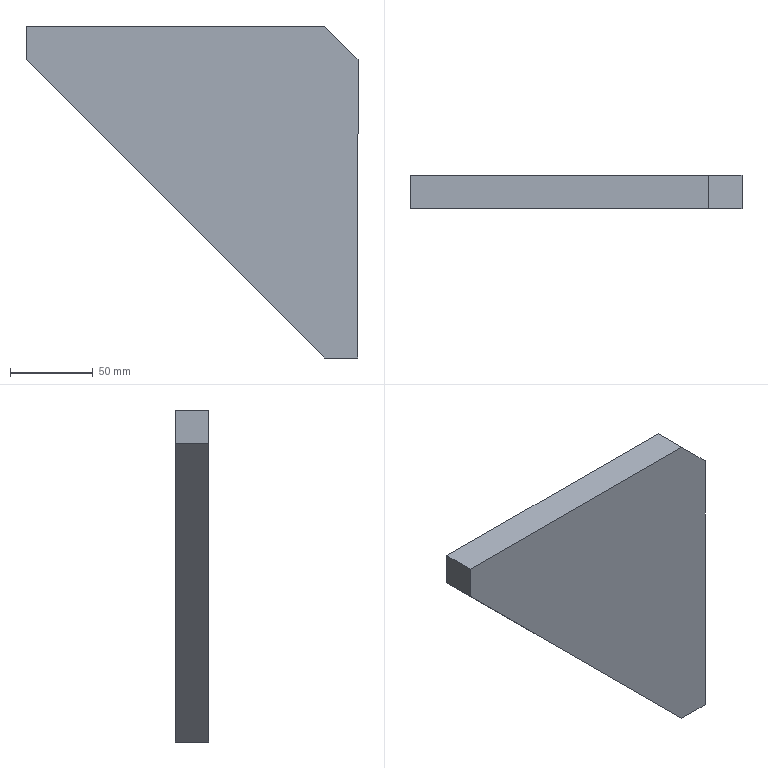Part | SolidWorks | features Extrusion 1 | 1 solid | 8 faces | box 200 x 20 x 200 mm | volume 472000 mm3 | plane 8
STEP:
#1=CARTESIAN_POINT('',(0.,0.,0.));
#2=VERTEX_POINT('',#1);
#3=CARTESIAN_POINT('',(-20.,0.,0.));
#4=VERTEX_POINT('',#3);
#5=CARTESIAN_POINT('',(-20.,0.,0.));
#6=DIRECTION('',(-1.,0.,0.));
#7=VECTOR('',#6,1000.);
#8=LINE('',#5,#7);
#9=EDGE_CURVE('',#2,#4,#8,.T.);
#10=ORIENTED_EDGE('',*,*,#9,.T.);
#11=CARTESIAN_POINT('',(-20.,20.,0.));
#12=VERTEX_POINT('',#11);
#13=CARTESIAN_POINT('',(-20.,20.,0.));
#14=DIRECTION('',(0.,-1.,0.));
#15=VECTOR('',#14,1000.);
#16=LINE('',#13,#15);
#17=EDGE_CURVE('',#12,#4,#16,.T.);
#18=ORIENTED_EDGE('',*,*,#17,.F.);
#19=CARTESIAN_POINT('',(0.,20.,0.));
#20=VERTEX_POINT('',#19);
#21=CARTESIAN_POINT('',(-20.,20.,0.));
#22=DIRECTION('',(-1.,0.,0.));
#23=VECTOR('',#22,1000.);
#24=LINE('',#21,#23);
#25=EDGE_CURVE('',#20,#12,#24,.T.);
#26=ORIENTED_EDGE('',*,*,#25,.F.);
#27=CARTESIAN_POINT('',(0.,20.,0.));
#28=DIRECTION('',(0.,-1.,0.));
#29=VECTOR('',#28,1000.);
#30=LINE('',#27,#29);
#31=EDGE_CURVE('',#20,#2,#30,.T.);
#32=ORIENTED_EDGE('',*,*,#31,.T.);
#33=EDGE_LOOP('',(#10,#18,#26,#32));
#34=FACE_OUTER_BOUND('',#33,.T.);
#35=CARTESIAN_POINT('',(-20.,20.,0.));
#36=DIRECTION('',(0.,0.,1.));
#37=DIRECTION('',(1.,0.,0.));
#38=AXIS2_PLACEMENT_3D('',#35,#36,#37);
#39=PLANE('',#38);
#40=ADVANCED_FACE('',(#34),#39,.F.);
#41=CARTESIAN_POINT('',(-200.,0.,180.));
#42=VERTEX_POINT('',#41);
#43=CARTESIAN_POINT('',(-200.,0.,180.));
#44=DIRECTION('',(-0.7071,0.,0.7071));
#45=VECTOR('',#44,1000.);
#46=LINE('',#43,#45);
#47=EDGE_CURVE('',#4,#42,#46,.T.);
#48=ORIENTED_EDGE('',*,*,#47,.T.);
#49=CARTESIAN_POINT('',(-200.,20.,180.));
#50=VERTEX_POINT('',#49);
#51=CARTESIAN_POINT('',(-200.,20.,180.));
#52=DIRECTION('',(0.,-1.,0.));
#53=VECTOR('',#52,1000.);
#54=LINE('',#51,#53);
#55=EDGE_CURVE('',#50,#42,#54,.T.);
#56=ORIENTED_EDGE('',*,*,#55,.F.);
#57=CARTESIAN_POINT('',(-200.,20.,180.));
#58=DIRECTION('',(-0.7071,0.,0.7071));
#59=VECTOR('',#58,1000.);
#60=LINE('',#57,#59);
#61=EDGE_CURVE('',#12,#50,#60,.T.);
#62=ORIENTED_EDGE('',*,*,#61,.F.);
#63=ORIENTED_EDGE('',*,*,#17,.T.);
#64=EDGE_LOOP('',(#48,#56,#62,#63));
#65=FACE_OUTER_BOUND('',#64,.T.);
#66=CARTESIAN_POINT('',(-200.,20.,180.));
#67=DIRECTION('',(0.7071,0.,0.7071));
#68=DIRECTION('',(0.7071,0.,-0.7071));
#69=AXIS2_PLACEMENT_3D('',#66,#67,#68);
#70=PLANE('',#69);
#71=ADVANCED_FACE('',(#65),#70,.F.);
#72=CARTESIAN_POINT('',(-200.,0.,200.));
#73=VERTEX_POINT('',#72);
#74=CARTESIAN_POINT('',(-200.,0.,200.));
#75=DIRECTION('',(0.,0.,1.));
#76=VECTOR('',#75,1000.);
#77=LINE('',#74,#76);
#78=EDGE_CURVE('',#42,#73,#77,.T.);
#79=ORIENTED_EDGE('',*,*,#78,.T.);
#80=CARTESIAN_POINT('',(-200.,20.,200.));
#81=VERTEX_POINT('',#80);
#82=CARTESIAN_POINT('',(-200.,20.,200.));
#83=DIRECTION('',(0.,-1.,0.));
#84=VECTOR('',#83,1000.);
#85=LINE('',#82,#84);
#86=EDGE_CURVE('',#81,#73,#85,.T.);
#87=ORIENTED_EDGE('',*,*,#86,.F.);
#88=CARTESIAN_POINT('',(-200.,20.,200.));
#89=DIRECTION('',(0.,0.,1.));
#90=VECTOR('',#89,1000.);
#91=LINE('',#88,#90);
#92=EDGE_CURVE('',#50,#81,#91,.T.);
#93=ORIENTED_EDGE('',*,*,#92,.F.);
#94=ORIENTED_EDGE('',*,*,#55,.T.);
#95=EDGE_LOOP('',(#79,#87,#93,#94));
#96=FACE_OUTER_BOUND('',#95,.T.);
#97=CARTESIAN_POINT('',(-200.,20.,200.));
#98=DIRECTION('',(1.,0.,0.));
#99=DIRECTION('',(0.,0.,-1.));
#100=AXIS2_PLACEMENT_3D('',#97,#98,#99);
#101=PLANE('',#100);
#102=ADVANCED_FACE('',(#96),#101,.F.);
#103=CARTESIAN_POINT('',(-20.,0.,200.));
#104=VERTEX_POINT('',#103);
#105=CARTESIAN_POINT('',(-20.,0.,200.));
#106=DIRECTION('',(1.,0.,0.));
#107=VECTOR('',#106,1000.);
#108=LINE('',#105,#107);
#109=EDGE_CURVE('',#73,#104,#108,.T.);
#110=ORIENTED_EDGE('',*,*,#109,.T.);
#111=CARTESIAN_POINT('',(-20.,20.,200.));
#112=VERTEX_POINT('',#111);
#113=CARTESIAN_POINT('',(-20.,20.,200.));
#114=DIRECTION('',(0.,-1.,0.));
#115=VECTOR('',#114,1000.);
#116=LINE('',#113,#115);
#117=EDGE_CURVE('',#112,#104,#116,.T.);
#118=ORIENTED_EDGE('',*,*,#117,.F.);
#119=CARTESIAN_POINT('',(-20.,20.,200.));
#120=DIRECTION('',(1.,0.,0.));
#121=VECTOR('',#120,1000.);
#122=LINE('',#119,#121);
#123=EDGE_CURVE('',#81,#112,#122,.T.);
#124=ORIENTED_EDGE('',*,*,#123,.F.);
#125=ORIENTED_EDGE('',*,*,#86,.T.);
#126=EDGE_LOOP('',(#110,#118,#124,#125));
#127=FACE_OUTER_BOUND('',#126,.T.);
#128=CARTESIAN_POINT('',(-20.,20.,200.));
#129=DIRECTION('',(0.,0.,-1.));
#130=DIRECTION('',(-1.,0.,0.));
#131=AXIS2_PLACEMENT_3D('',#128,#129,#130);
#132=PLANE('',#131);
#133=ADVANCED_FACE('',(#127),#132,.F.);
#134=CARTESIAN_POINT('',(0.,0.,180.));
#135=VERTEX_POINT('',#134);
#136=CARTESIAN_POINT('',(0.,0.,180.));
#137=DIRECTION('',(0.7071,0.,-0.7071));
#138=VECTOR('',#137,1000.);
#139=LINE('',#136,#138);
#140=EDGE_CURVE('',#104,#135,#139,.T.);
#141=ORIENTED_EDGE('',*,*,#140,.T.);
#142=CARTESIAN_POINT('',(0.,20.,180.));
#143=VERTEX_POINT('',#142);
#144=CARTESIAN_POINT('',(0.,20.,180.));
#145=DIRECTION('',(0.,-1.,0.));
#146=VECTOR('',#145,1000.);
#147=LINE('',#144,#146);
#148=EDGE_CURVE('',#143,#135,#147,.T.);
#149=ORIENTED_EDGE('',*,*,#148,.F.);
#150=CARTESIAN_POINT('',(0.,20.,180.));
#151=DIRECTION('',(0.7071,0.,-0.7071));
#152=VECTOR('',#151,1000.);
#153=LINE('',#150,#152);
#154=EDGE_CURVE('',#112,#143,#153,.T.);
#155=ORIENTED_EDGE('',*,*,#154,.F.);
#156=ORIENTED_EDGE('',*,*,#117,.T.);
#157=EDGE_LOOP('',(#141,#149,#155,#156));
#158=FACE_OUTER_BOUND('',#157,.T.);
#159=CARTESIAN_POINT('',(0.,20.,180.));
#160=DIRECTION('',(-0.7071,0.,-0.7071));
#161=DIRECTION('',(-0.7071,0.,0.7071));
#162=AXIS2_PLACEMENT_3D('',#159,#160,#161);
#163=PLANE('',#162);
#164=ADVANCED_FACE('',(#158),#163,.F.);
#165=CARTESIAN_POINT('',(0.,0.,0.));
#166=DIRECTION('',(0.,0.,-1.));
#167=VECTOR('',#166,1000.);
#168=LINE('',#165,#167);
#169=EDGE_CURVE('',#135,#2,#168,.T.);
#170=ORIENTED_EDGE('',*,*,#169,.T.);
#171=ORIENTED_EDGE('',*,*,#31,.F.);
#172=CARTESIAN_POINT('',(0.,20.,0.));
#173=DIRECTION('',(0.,0.,-1.));
#174=VECTOR('',#173,1000.);
#175=LINE('',#172,#174);
#176=EDGE_CURVE('',#143,#20,#175,.T.);
#177=ORIENTED_EDGE('',*,*,#176,.F.);
#178=ORIENTED_EDGE('',*,*,#148,.T.);
#179=EDGE_LOOP('',(#170,#171,#177,#178));
#180=FACE_OUTER_BOUND('',#179,.T.);
#181=CARTESIAN_POINT('',(0.,20.,0.));
#182=DIRECTION('',(-1.,0.,0.));
#183=DIRECTION('',(0.,0.,1.));
#184=AXIS2_PLACEMENT_3D('',#181,#182,#183);
#185=PLANE('',#184);
#186=ADVANCED_FACE('',(#180),#185,.F.);
#187=ORIENTED_EDGE('',*,*,#25,.T.);
#188=ORIENTED_EDGE('',*,*,#61,.T.);
#189=ORIENTED_EDGE('',*,*,#92,.T.);
#190=ORIENTED_EDGE('',*,*,#123,.T.);
#191=ORIENTED_EDGE('',*,*,#154,.T.);
#192=ORIENTED_EDGE('',*,*,#176,.T.);
#193=EDGE_LOOP('',(#187,#188,#189,#190,#191,#192));
#194=FACE_OUTER_BOUND('',#193,.T.);
#195=CARTESIAN_POINT('',(0.,20.,0.));
#196=DIRECTION('',(0.,-1.,0.));
#197=DIRECTION('',(0.,0.,-1.));
#198=AXIS2_PLACEMENT_3D('',#195,#196,#197);
#199=PLANE('',#198);
#200=ADVANCED_FACE('',(#194),#199,.F.);
#201=ORIENTED_EDGE('',*,*,#9,.F.);
#202=ORIENTED_EDGE('',*,*,#169,.F.);
#203=ORIENTED_EDGE('',*,*,#140,.F.);
#204=ORIENTED_EDGE('',*,*,#109,.F.);
#205=ORIENTED_EDGE('',*,*,#78,.F.);
#206=ORIENTED_EDGE('',*,*,#47,.F.);
#207=EDGE_LOOP('',(#201,#202,#203,#204,#205,#206));
#208=FACE_OUTER_BOUND('',#207,.T.);
#209=CARTESIAN_POINT('',(0.,0.,0.));
#210=DIRECTION('',(0.,-1.,0.));
#211=DIRECTION('',(0.,0.,-1.));
#212=AXIS2_PLACEMENT_3D('',#209,#210,#211);
#213=PLANE('',#212);
#214=ADVANCED_FACE('',(#208),#213,.T.);
#215=CLOSED_SHELL('',(#40,#71,#102,#133,#164,#186,#200,#214));
#216=MANIFOLD_SOLID_BREP('',#215);
#217=CARTESIAN_POINT('',(0.,0.,0.));
#218=DIRECTION('',(0.,0.,1.));
#219=DIRECTION('',(1.,0.,0.));
#220=AXIS2_PLACEMENT_3D('',#217,#218,#219);
#221=(LENGTH_UNIT()NAMED_UNIT(*)SI_UNIT(.MILLI.,.METRE.));
#222=UNCERTAINTY_MEASURE_WITH_UNIT(LENGTH_MEASURE(0.00001),#221,'','');
#223=(NAMED_UNIT(*)PLANE_ANGLE_UNIT()SI_UNIT($,.RADIAN.));
#224=(NAMED_UNIT(*)SI_UNIT($,.STERADIAN.)SOLID_ANGLE_UNIT());
#225=(GEOMETRIC_REPRESENTATION_CONTEXT(3)GLOBAL_UNCERTAINTY_ASSIGNED_CONTEXT((#222))GLOBAL_UNIT_ASSIGNED_CONTEXT((#221,#223,#224))REPRESENTATION_CONTEXT('',''));
#226=ADVANCED_BREP_SHAPE_REPRESENTATION('',(#216,#220),#225);